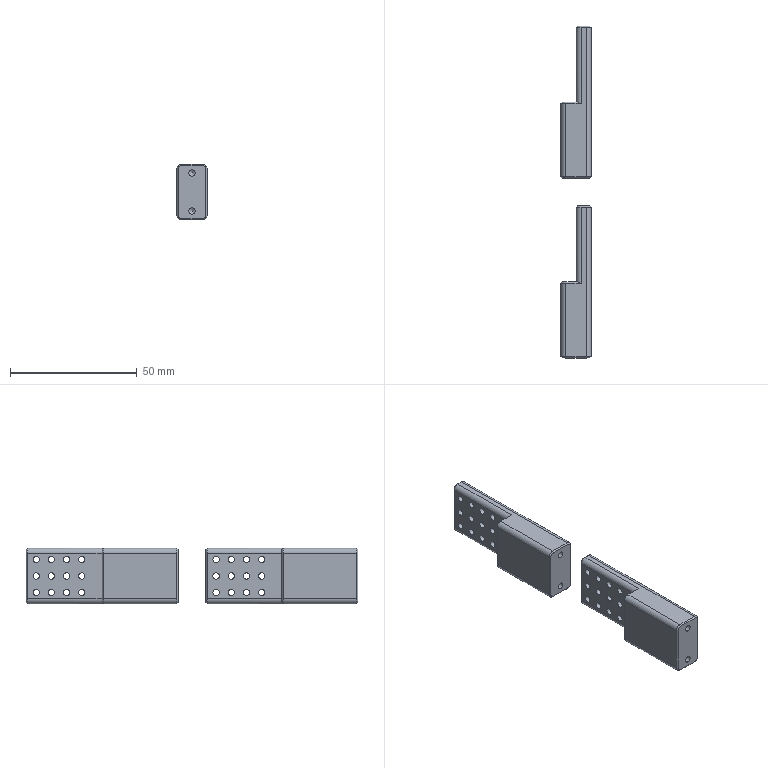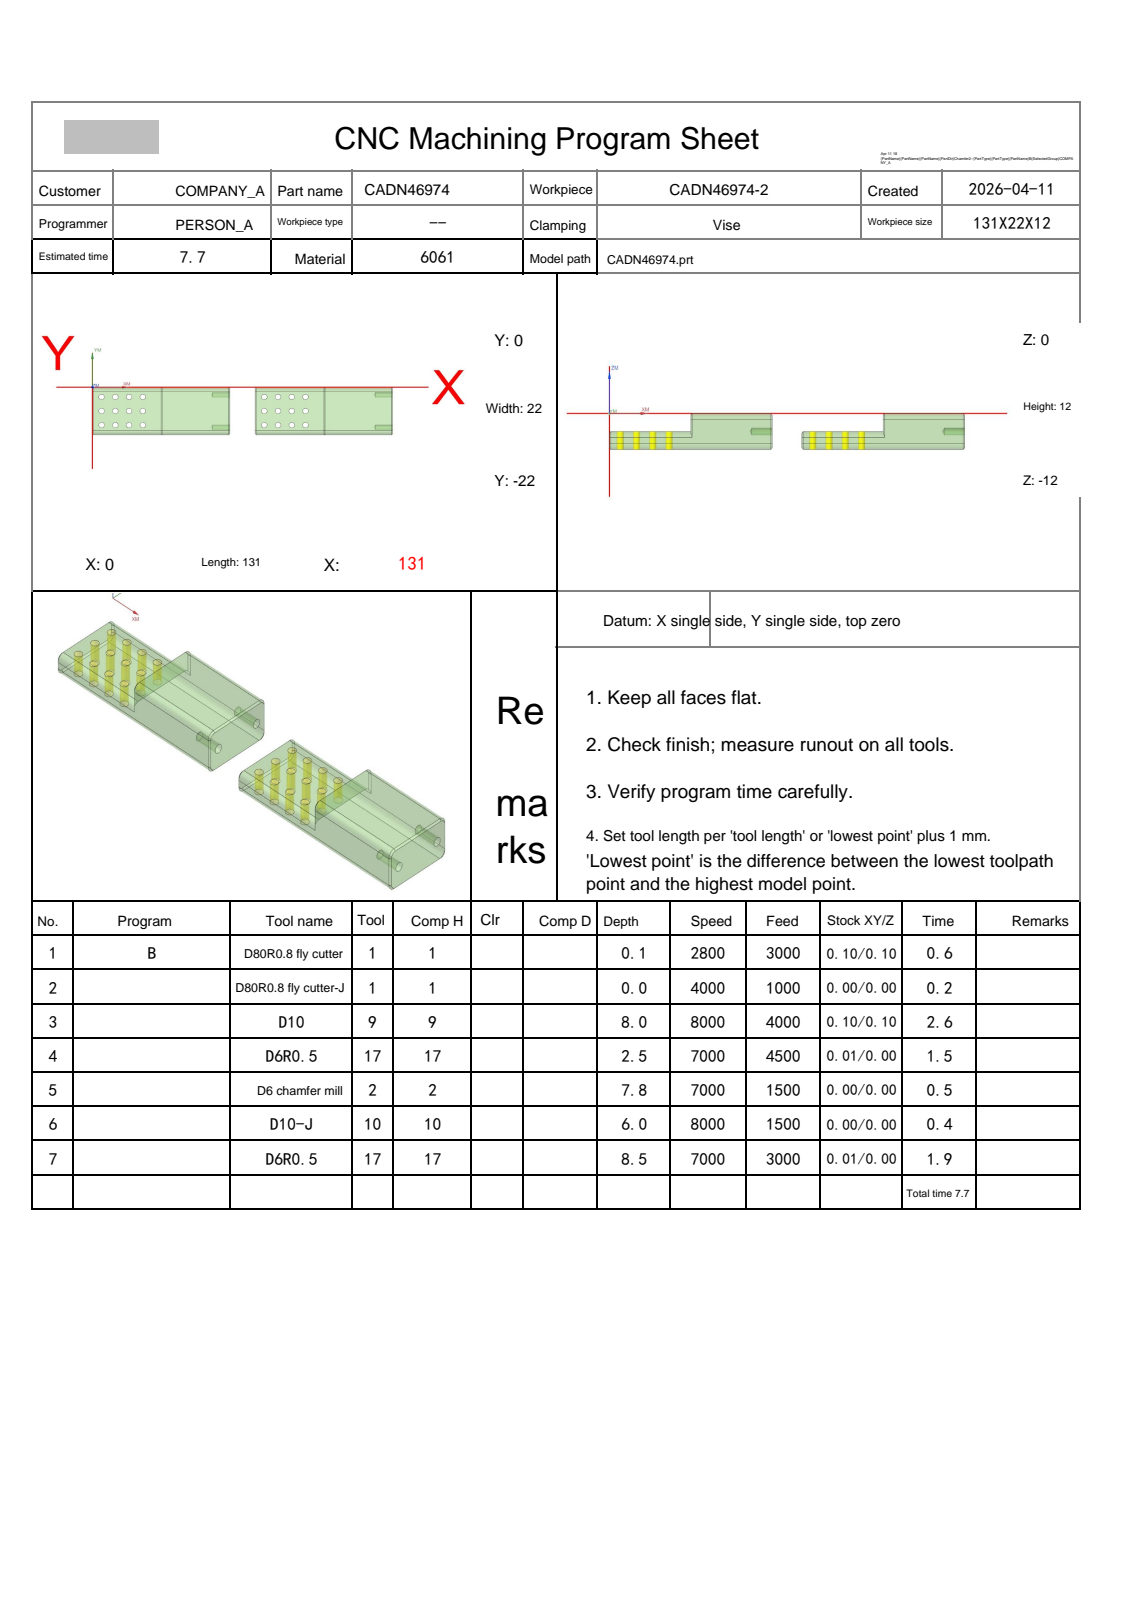NC program | NX | posted by the shop | part box 12 x 131 x 22 mm
Lines 2208 to 4050 of 5054, first 1531 of 1843 lines:
N4 T17 M06
(D6R0.5  D=6. R=0.5 H=17 ce=0.01 di=0.00)
G00 G90 G54 X134.304 Y-17.731 M03 S7000
G43 H17 Z12.8
M08
Z.491
G01 Z-.009 F4500.
X134.298
G03 X133.098 Y-18.901 I0.0 J-1.2
G01 X133.062 Y-20.314
X133.057 Y-20.363
G02 X130.5 Y-22.721 I-2.634 J.291
G01 X101.5
G02 X98.936 Y-20.411 I.115 J2.706
G01 X98.922 Y-20.314
X98.9 Y-18.897
X98.868 Y-18.899 Z-.015
X98.852 Y-18.9 Z-.021
X98.866 Y-20.229
G03 X101.5 Y-22.836 I2.634 J.027
G01 X130.5
G03 X133.136 Y-20.123 I-.105 J2.739
G01 X133.148 Y-18.824
X133.2 Y-18.862 Z-.038
G02 X133.221 Y-19.445 I-7.917 J-.583
X133.119 Y-20.718 I-7.939 J0.0
X130.503 Y-22.943 I-2.616 J.425
G01 X101.5
G02 X98.835 Y-20.462 I.099 J2.778
G01 X98.815 Y-20.314
X98.802 Y-18.898
X98.776 Y-18.9 Z-.048
X98.761 Y-18.901 Z-.058
X98.774 Y-20.314
X98.806 Y-20.574
G03 X101.5 Y-23.046 I2.795 J.343
G01 X130.5
G03 X133.183 Y-20.659 I-.1 J2.813
G01 X133.227 Y-20.314
X133.239 Y-18.893
X133.284 Y-18.849 Z-.082
G02 X133.307 Y-19.453 I-7.772 J-.604
X133.185 Y-20.829 I-7.795 J0.0
X130.5 Y-23.147 I-2.772 J.497
G01 X101.5
G02 X98.773 Y-20.659 I.093 J2.84
G01 X98.729 Y-20.314
X98.717 Y-18.898
X98.695 Y-18.899 Z-.096
X98.682 Z-.111
X98.691 Y-20.217
G03 X98.884 Y-21.265 I3.067 J.022
G01 X98.979 Y-21.52
G03 X101.5 Y-23.245 I2.589 J1.078
G01 X130.5
X131.427 Y-23.074
G03 X133.307 Y-20.314 I-1.159 J2.809
G01 X133.321 Y-18.887
X133.358 Y-18.914 Z-.143
X133.341 Y-20.314
X133.309 Y-20.659
G02 X131.734 Y-23.033 I-3.07 J.327
X130.5 Y-23.342 I-1.431 J3.097
G01 X101.499
G02 X99.343 Y-22.252 I0.0 J2.678
X98.654 Y-20.314 I2.867 J2.111
G01 X98.642 Y-18.9
X98.605 Y-18.892 Z-.178
X98.614 Y-20.143
G03 X98.98 Y-21.785 I4.005 J.03
X101.5 Y-23.437 I2.578 J1.184
G01 X130.542
G03 X132.379 Y-22.673 I0.0 J2.591
X133.379 Y-20.314 I-2.438 J2.424
G01 X133.395 Y-18.879
X133.435 Y-18.87 Z-.218
X133.42 Y-20.314
X133.385 Y-20.659
G02 X132.434 Y-22.729 I-3.452 J.333
X130.5 Y-23.53 I-1.994 J2.08
G01 X101.5
G02 X99.052 Y-22.039 I.043 J2.826
X98.575 Y-20.171 I3.544 J1.899
G01 X98.565 Y-18.893
X98.522 Y-18.895 Z-.261
Y-19.969
Y-19.986
G03 X98.983 Y-22.039 I4.81 J0.0
X101.5 Y-23.622 I2.57 J1.295
G01 X130.5
G03 X133.008 Y-22.039 I-.042 J2.846
X133.466 Y-20.314 I-3.959 J1.972
G01 X133.478 Y-18.895
X133.524 Y-18.896 Z-.307
X133.512 Y-20.314
X133.476 Y-20.659
G02 X132.873 Y-22.384 I-4.307 J.538
X130.5 Y-23.711 I-2.397 J1.502
G01 X101.5
G02 X98.979 Y-22.133 I.036 J2.86
X98.476 Y-19.978 I4.359 J2.154
G01 Y-19.969
Y-18.896
X98.425 Y-18.897 Z-.357
Y-19.969
G03 X99.063 Y-22.384 I4.888 J0.0
X101.5 Y-23.798 I2.461 J1.435
G01 X130.5
G03 X132.945 Y-22.384 I-.043 J2.894
X133.575 Y-19.969 I-4.383 J2.433
G01 Y-18.897
X133.628 Y-18.899 Z-.411
G02 X133.636 Y-19.434 I-17.574 J-.535
X133.623 Y-20.105 I-17.582 J0.0
X132.993 Y-22.39 I-5.175 J.198
X130.5 Y-23.883 I-2.517 J1.375
G01 X101.5
G02 X98.995 Y-22.379 I.033 J2.893
X98.382 Y-20.029 I4.383 J2.398
G01 X98.372 Y-18.934
Y-18.899
X98.315 Y-18.901 Z-.468
G03 X98.307 Y-19.433 I17.643 J-.533
X98.321 Y-20.132 I17.651 J0.0
X99.153 Y-22.729 I5.098 J.202
X101.5 Y-23.966 I2.378 J1.667
G01 X130.5
G03 X132.939 Y-22.592 I-.037 J2.917
G01 X133.052 Y-22.384
G03 X133.665 Y-20.325 I-4.423 J2.438
X133.698 Y-19.448 I-11.669 J.877
X133.685 Y-18.901 I-11.702 J0.0
G01 X133.745 Y-18.902 Z-.528
G02 X133.758 Y-19.447 I-11.605 J-.544
X133.729 Y-20.266 I-11.618 J0.0
X132.912 Y-22.719 I-5.196 J.367
X130.5 Y-24.047 I-2.435 J1.568
G01 X101.5
G02 X99.097 Y-22.729 I.02 J2.886
X98.305 Y-20.659 I4.593 J2.943
X98.242 Y-19.439 I11.682 J1.22
X98.255 Y-18.888 I11.745 J0.0
G01 X98.192 Y-18.895 Z-.591
G03 X98.184 Y-19.367 I13.801 J-.472
X98.244 Y-20.659 I13.809 J0.0
X99.134 Y-22.873 I5.506 J.927
X101.498 Y-24.125 I2.365 J1.609
G01 X130.502
G03 X132.851 Y-22.893 I0.0 J2.856
X133.757 Y-20.659 I-4.549 J3.146
X133.821 Y-19.437 I-11.656 J1.222
X133.808 Y-18.895 I-11.72 J0.0
G01 X133.874 Y-18.857 Z-.658
G02 X133.882 Y-19.35 I-14.17 J-.493
X133.822 Y-20.659 I-14.179 J0.0
X133.016 Y-22.729 I-5.538 J.965
G01 X132.783 Y-23.074
G02 X130.5 Y-24.2 I-2.308 J1.802
G01 X101.5
G02 X99.221 Y-23.074 I.016 J2.902
X98.18 Y-20.659 I4.483 J3.364
X98.118 Y-19.371 I13.177 J1.288
X98.126 Y-18.893 I13.24 J0.0
G01 X98.06 Y-18.873 Z-.727
G03 X98.049 Y-19.388 I12.491 J-.515
X98.114 Y-20.659 I12.502 J0.0
X98.979 Y-22.807 I5.655 J1.029
G01 X99.153 Y-23.074
G03 X101.5 Y-24.272 I2.375 J1.755
G01 X130.503
G03 X132.896 Y-22.989 I0.0 J2.874
G01 X133.069 Y-22.729
G03 X133.888 Y-20.659 I-4.561 J3.001
X133.95 Y-19.394 I-12.75 J1.266
X133.937 Y-18.818 I-12.813 J0.0
G01 X134.01 Y-18.851 Z-.798
G02 X134.021 Y-19.375 I-12.518 J-.524
X133.955 Y-20.659 I-12.529 J0.0
X133.114 Y-22.744 I-5.292 J.923
X131.746 Y-24.054 I-2.75 J1.503
X130.513 Y-24.341 I-1.233 J2.508
G01 X101.5
G02 X99.101 Y-23.074 I.02 J2.943
G01 X98.979 Y-22.886
X98.872 Y-22.729
G02 X98.046 Y-20.659 I4.544 J3.013
X97.979 Y-19.392 I11.911 J1.267
X97.993 Y-18.807 I11.978 J0.0
G01 X97.916 Y-18.922 Z-.868
G03 X97.908 Y-19.353 I12.331 J-.432
X97.978 Y-20.659 I12.339 J0.0
X98.979 Y-22.965 I5.452 J.997
X101.5 Y-24.404 I2.547 J1.533
G01 X130.512
G03 X132.403 Y-23.687 I0.0 J2.85
X133.177 Y-22.729 I-2.47 J2.787
X134.022 Y-20.659 I-4.327 J2.975
X134.091 Y-19.376 I-11.896 J1.283
X134.075 Y-18.762 I-11.965 J0.0
G01 X134.119 Y-18.843 Z-.904
X134.155 Y-18.924 Z-.939
X134.148 Y-19.969
G02 X133.631 Y-22.039 I-4.64 J.061
X132.773 Y-23.373 I-6.825 J3.448
X130.503 Y-24.463 I-2.27 J1.819
G01 X101.5
G02 X98.979 Y-23.044 I.038 J3.016
X97.91 Y-20.659 I4.625 J3.506
X97.838 Y-19.335 I12.252 J1.324
X97.845 Y-18.924 I12.324 J0.0
G01 X97.809 Y-18.925 Z-.974
X97.775 Y-18.926 Z-1.01
X97.781 Y-19.969
G03 X98.289 Y-22.007 I4.711 J.094
X99.212 Y-23.419 I7.675 J4.006
X101.5 Y-24.517 I2.303 J1.865
G01 X130.5
G03 X132.769 Y-23.442 I-.024 J2.981
X133.691 Y-22.039 I-6.854 J5.512
X134.219 Y-19.969 I-4.136 J2.156
G01 X134.226 Y-18.926
X134.261 Y-18.927 Z-1.045
X134.296 Y-18.928 Z-1.08
X134.289 Y-19.969
G02 X133.752 Y-22.039 I-4.66 J.105
X132.769 Y-23.495 I-8.012 J4.352
X130.5 Y-24.568 I-2.285 J1.895
G01 X101.495
G02 X99.253 Y-23.52 I0.0 J2.924
X98.289 Y-22.119 I6.943 J5.805
X97.712 Y-19.969 I4.069 J2.246
G01 X97.704 Y-18.928
X97.668 Y-18.929 Z-1.116
X97.633 Y-18.93 Z-1.151
X97.642 Y-19.969
G03 X98.19 Y-22.039 I4.546 J.095
X99.302 Y-23.621 I7.794 J4.297
X101.499 Y-24.615 I2.198 J1.934
G01 X130.5
G03 X132.769 Y-23.547 I-.023 J2.994
G01 X132.873 Y-23.419
G03 X133.803 Y-22.053 I-7.135 J5.857
X134.359 Y-19.969 I-4.069 J2.202
G01 X134.367 Y-18.93
X134.403 Y-18.931 Z-1.186
X134.438 Y-18.932 Z-1.222
X134.43 Y-19.969
G02 X133.868 Y-22.039 I-4.516 J.115
X132.616 Y-23.764 I-8.164 J4.607
X130.5 Y-24.659 I-2.143 J2.12
G01 X101.5
G02 X99.384 Y-23.764 I.021 J3.
X98.133 Y-22.039 I7.133 J6.49
X97.573 Y-19.969 I3.897 J2.165
G01 X97.562 Y-18.932
X97.527 Y-18.933 Z-1.257
X97.492 Y-18.934 Z-1.293
X97.503 Y-19.969
G03 X98.076 Y-22.039 I4.373 J.097
X99.408 Y-23.833 I8.913 J5.226
X101.048 Y-24.662 I2.114 J2.144
G01 X101.5 Y-24.699
X130.5
G03 X132.658 Y-23.764 I-.031 J3.03
X133.924 Y-22.039 I-7.483 J6.819
X134.5 Y-19.969 I-3.83 J2.181
G01 X134.509 Y-18.934
X134.543 Y-19.083 Z-1.328
X134.576 Y-19.231 Z-1.363
X134.571 Y-19.969
G02 X133.98 Y-22.039 I-4.306 J.11
X132.769 Y-23.676 I-8.71 J5.18
G01 X132.696 Y-23.764
G02 X131.045 Y-24.684 I-2.21 J2.023
G01 X130.5 Y-24.737
X101.5
X101.048 Y-24.701
G02 X99.306 Y-23.764 I.46 J2.943
X98.125 Y-22.219 I9.01 J8.108
X97.455 Y-20.277 I3.641 J2.344
X97.42 Y-19.527 I8.026 J.75
X97.425 Y-19.228 I8.061 J0.0
G01 X97.409 Y-19.397 Z-1.381
X97.393 Y-19.566 Z-1.399
X97.377 Y-19.734 Z-1.416
X97.363 Y-19.903 Z-1.434
G03 X97.945 Y-22.006 I4.116 J.007
X99.275 Y-23.764 I9.42 J5.749
G01 X99.324 Y-23.824
G03 X101.5 Y-24.771 I2.188 J2.052
G01 X130.5
G03 X132.728 Y-23.764 I-.014 J2.998
G01 X132.769 Y-23.715
G03 X134.036 Y-22.039 I-7.98 J7.352
X134.641 Y-19.922 I-3.575 J2.168
G01 X134.649 Y-20.076 Z-1.444
X134.646 Y-20.229 Z-1.455
X134.639 Y-20.383 Z-1.465
X134.63 Y-20.537 Z-1.476
X134.614 Y-20.69 Z-1.486
X134.59 Y-20.84 Z-1.496
X134.559 Y-20.988 Z-1.507
G02 X134.094 Y-22.039 I-4.048 J1.163
X132.595 Y-23.936 I-10.144 J6.475
X130.5 Y-24.804 I-2.104 J2.115
G01 X101.5
G02 X99.301 Y-23.833 I.013 J3.004
G01 X99.244 Y-23.764
G02 X97.945 Y-22.101 I8.56 J8.028
X97.441 Y-20.991 I3.59 J2.297
G01 X97.462 Y-21.129 Z-1.526
X97.49 Y-21.264 Z-1.545
X97.527 Y-21.397 Z-1.565
X97.571 Y-21.525 Z-1.584
G03 X97.945 Y-22.196 I3.829 J1.693
X98.902 Y-23.419 I10.343 J7.104
G01 X99.211 Y-23.764
X99.268 Y-23.833
G03 X101.5 Y-24.836 I2.243 J2.008
G01 X130.5
G03 X132.612 Y-23.954 I-.008 J2.986
X134.148 Y-22.049 I-9.472 J9.214
X134.43 Y-21.521 I-2.751 J1.811
G01 X134.402 Y-21.64 Z-1.611
X134.366 Y-21.757 Z-1.639
X134.316 Y-21.865 Z-1.666
X134.148 Y-22.148
G02 X132.63 Y-23.973 I-13.4 J9.608
X130.5 Y-24.867 I-2.14 J2.115
G01 X101.495
G02 X99.378 Y-23.976 I0.0 J2.959
X97.945 Y-22.278 I11.005 J10.749
X97.68 Y-21.866 I2.727 J2.042
G01 X97.719 Y-21.994 Z-1.709
X97.771 Y-22.114 Z-1.751
G03 X99.04 Y-23.651 I11.128 J7.893
G01 X99.28 Y-23.902
X99.324 Y-23.957
G03 X101.5 Y-24.895 I2.194 J2.095
G01 X130.501
G03 X132.7 Y-23.926 I0.0 J2.981
G01 X132.769 Y-23.852
G03 X134.226 Y-22.12 I-11.388 J11.064
G01 X134.19 Y-22.222 Z-1.796
X134.146 Y-22.317 Z-1.84
G02 X132.769 Y-23.879 I-16.258 J12.952
G01 X132.658 Y-24.001
G02 X130.5 Y-24.921 I-2.167 J2.092
G01 X101.5
G02 X99.311 Y-23.971 I.008 J3.014
G01 X99.254 Y-23.902
G02 X97.849 Y-22.304 I11.657 J11.671
G01 X97.914 Y-22.46 Z-1.931
G03 X99.227 Y-23.902 I22.34 J19.019
G01 X99.288 Y-23.971
G03 X101.5 Y-24.944 I2.221 J2.048
G01 X130.5
G03 X132.671 Y-24.015 I-.016 J3.036
G01 X132.769 Y-23.906
G03 X134.099 Y-22.444 I-20.932 J20.375
G01 X134.058 Y-22.542 Z-2.025
G02 X132.68 Y-24.025 I-27.765 J24.408
X130.5 Y-24.964 I-2.186 J2.072
G01 X101.5
G02 X99.334 Y-24.04 I.004 J3.008
X97.96 Y-22.569 I34.655 J33.753
G01 X97.997 Y-22.654 Z-2.121
G03 X99.384 Y-24.109 I47.473 J43.852
X101.5 Y-24.981 I2.122 J2.145
G01 X130.503
G03 X132.631 Y-24.093 I0.0 J2.994
X134.011 Y-22.638 I-34.23 J33.868
G01 X133.963 Y-22.729 Z-2.216
G02 X132.58 Y-24.158 I-81.21 J77.228
X130.5 Y-24.994 I-2.097 J2.213
G01 X101.5
G02 X99.303 Y-24.04 I.013 J3.036
G01 X98.036 Y-22.731
X98.044 Y-22.762 Z-2.311
X99.376 Y-24.122
G03 X99.925 Y-24.556 I1.98 J1.94
X101.5 Y-25.003 I1.607 J2.664
G01 X130.5
G03 X132.587 Y-24.158 I-.018 J3.045
G01 X132.769 Y-23.972
X133.949 Y-22.765
X133.933 Y-22.798 Z-2.405
X132.636 Y-24.116
G02 X130.506 Y-25.008 I-2.13 J2.097
G01 X101.499
G02 X99.362 Y-24.114 I0.0 J3.001
G01 X98.289 Y-23.027
X98.056 Y-22.789
X98.069 Y-22.815 Z-2.5
X98.289 Y-23.041
X99.352 Y-24.109
G03 X101.5 Y-25.01 I2.149 J2.112
G01 X130.5
G03 X132.598 Y-24.158 I0.0 J3.01
G01 X132.769 Y-23.988
X133.917 Y-22.831
G00 Z12.8
X97.696 Y-4.284
Z.491
G01 Z-.009
X97.7
G03 X98.9 Y-3.103 I0.0 J1.2
G01 X98.922 Y-1.686
X98.936 Y-1.589
G02 X101.5 Y.721 I2.679 J-.396
G01 X130.5
G02 X133.041 Y-1.768 I-.05 J-2.593
G01 X133.1 Y-3.238
X133.148 Y-3.1 Z-.021
X133.136 Y-1.877
G03 X130.5 Y.836 I-2.741 J-.027
G01 X101.5
G03 X98.881 Y-1.545 I.08 J-2.719
G01 X98.867 Y-1.686
X98.852 Y-3.099
X98.801 Y-3.1 Z-.038
X98.815 Y-1.686
X98.835 Y-1.538
G02 X101.5 Y.943 I2.764 J-.297
G01 X130.505
G02 X133.117 Y-1.274 I0.0 J-2.648
X133.221 Y-2.536 I-7.65 J-1.263
X133.2 Y-3.1 I-7.753 J0.0
G01 X133.223 Z-.048
X133.239 Z-.058
X133.227 Y-1.686
X133.183 Y-1.341
G03 X130.5 Y1.046 I-2.783 J-.427
G01 X101.5
G03 X98.804 Y-1.436 I.111 J-2.826
G01 X98.774 Y-1.686
X98.761 Y-3.099
X98.734 Y-3.1 Z-.07
X98.717 Y-3.102 Z-.082
X98.729 Y-1.686
X98.773 Y-1.341
G02 X101.5 Y1.147 I2.819 J-.352
G01 X130.5
G02 X133.184 Y-1.161 I-.087 J-2.816
X133.307 Y-2.516 I-7.385 J-1.356
X133.285 Y-3.1 I-7.508 J0.0
G01 X133.321 Z-.111
X133.307 Y-1.686
X133.271 Y-1.341
G03 X130.5 Y1.245 I-2.885 J-.314
G01 X101.5
G03 X100.013 Y.781 I.106 J-2.953
X98.719 Y-1.424 I1.776 J-2.524
G01 X98.692 Y-1.686
X98.682 Y-3.101
X98.658 Y-3.1 Z-.127
X98.642 Z-.143
X98.654 Y-1.686
X98.687 Y-1.341
G02 X100.358 Y1.084 I3.104 J-.351
X101.5 Y1.342 I1.417 J-3.623
G01 X130.5
G02 X132.813 Y.039 I-.062 J-2.815
G01 X132.938 Y-.191
G02 X133.341 Y-1.742 I-2.947 J-1.595
G01 X133.359 Y-3.1
X133.395 Y-3.121 Z-.178
X133.379 Y-1.686
G03 X132.883 Y.039 I-3.682 J-.123
X130.5 Y1.437 I-2.445 J-1.438
G01 X101.5
G03 X99.673 Y.729 I.087 J-2.938
X98.65 Y-1.341 I2.328 J-2.438
G01 X98.615 Y-1.686
X98.605 Y-3.108
X98.565 Y-3.107 Z-.218
X98.576 Y-1.686
X98.613 Y-1.341
G02 X99.221 Y.31 I3.757 J-.447
X101.5 Y1.53 I2.279 J-1.518
G01 X130.5
G02 X133.12 Y-.306 I-.063 J-2.878
X133.433 Y-1.992 I-4.391 J-1.686
G01 Y-2.031
X133.435 Y-3.13
X133.478 Y-3.106 Z-.261
X133.466 Y-1.686
G03 X133.008 Y.039 I-4.416 J-.247
X130.5 Y1.622 I-2.55 J-1.263
G01 X101.5
G03 X98.983 Y.039 I.052 J-2.877
X98.532 Y-1.904 I4.126 J-1.981
G01 X98.522 Y-3.105
X98.499 Z-.284
X98.476 Y-3.104 Z-.307
X98.486 Y-1.917
G02 X98.976 Y.127 I4.67 J-.04
X101.5 Y1.711 I2.56 J-1.276
G01 X130.5
G02 X133.067 Y.039 I-.037 J-2.865
X133.524 Y-2.027 I-4.442 J-2.066
G01 Y-2.031
Y-3.105
X133.575 Y-3.103 Z-.357
Y-2.031
G03 X132.945 Y.384 I-5.013 J-.018
X130.5 Y1.798 I-2.487 J-1.48
G01 X101.5
G03 X99.063 Y.384 I.024 J-2.849
X98.438 Y-1.686 I4.231 J-2.407
G01 X98.425 Y-3.103
X98.399 Y-3.102 Z-.384
X98.372 Y-3.101 Z-.411
G02 X98.364 Y-2.566 I18.376 J.535
X98.378 Y-1.861 I18.384 J0.0
X98.992 Y.374 I5.078 J-.195
X101.5 Y1.883 I2.541 J-1.383
G01 X130.5
G02 X132.993 Y.39 I-.024 J-2.868
X133.623 Y-1.897 I-4.546 J-2.483
X133.636 Y-2.568 I-17.763 J-.671
X133.628 Y-3.102 I-17.776 J0.0
G01 X133.685 Y-3.1 Z-.468
G03 X133.698 Y-2.55 I-11.598 J.55
X133.665 Y-1.67 I-11.611 J0.0
X133.069 Y.352 I-5.028 J-.382
G01 X132.939 Y.592
G03 X130.5 Y1.966 I-2.476 J-1.542
G01 X101.5
G03 X99.153 Y.729 I.031 J-2.904
X98.321 Y-1.866 I4.267 J-2.799
X98.307 Y-2.565 I17.476 J-.699
X98.315 Y-3.099 I17.49 J0.0
G01 X98.255 Y-3.112 Z-.528
G02 X98.242 Y-2.566 I11.922 J.545
X98.305 Y-1.341 I11.935 J0.0
X99.097 Y.729 I5.385 J-.873
X101.5 Y2.047 I2.423 J-1.569
G01 X130.5
G02 X132.912 Y.719 I-.022 J-2.896
X133.729 Y-1.732 I-4.382 J-2.822
X133.758 Y-2.55 I-11.474 J-.818
X133.745 Y-3.098 I-11.503 J0.0
G01 X133.808 Y-3.105 Z-.591
G03 X133.822 Y-2.557 I-11.482 J.549
X133.757 Y-1.341 I-11.495 J0.0
X132.851 Y.893 I-5.455 J-.913
X130.502 Y2.125 I-2.349 J-1.625
G01 X101.499
G03 X99.133 Y.873 I0.0 J-2.86
X98.244 Y-1.341 I4.618 J-3.141
X98.184 Y-2.636 I13.839 J-1.295
X98.192 Y-3.105 I13.899 J0.0
G01 X98.126 Y-3.085 Z-.658
G02 X98.118 Y-2.627 I13.249 J.458
X98.18 Y-1.341 I13.257 J0.0
X99.221 Y1.074 I5.526 J-.951
X101.5 Y2.2 I2.295 J-1.776
G01 X130.5
G02 X132.783 Y1.074 I-.025 J-2.928
G01 X132.948 Y.83
G02 X133.822 Y-1.341 I-4.634 J-3.127
X133.881 Y-2.632 I-13.939 J-1.291
X133.874 Y-3.086 I-13.999 J0.0
G01 X133.909 Y-3.085 Z-.692
X133.942 Y-3.084 Z-.727
G03 X133.95 Y-2.625 I-13.192 J.458
X133.888 Y-1.341 I-13.2 J0.0
X133.069 Y.729 I-5.378 J-.93
G01 X132.84 Y1.074
G03 X130.5 Y2.272 I-2.357 J-1.72
G01 X101.498
G03 X99.079 Y.961 I0.0 J-2.887
G01 X98.979 Y.807
G03 X98.114 Y-1.341 I4.793 J-3.179
X98.049 Y-2.627 I12.735 J-1.286
X98.057 Y-3.083 I12.799 J0.0
G01 X98.021 Y-3.082 Z-.762
X97.986 Y-3.081 Z-.798
G02 X97.978 Y-2.635 I12.478 J.446
X98.046 Y-1.341 I12.486 J0.0
X98.979 Y.886 I5.399 J-.954
X101.5 Y2.341 I2.545 J-1.498
G01 X130.5
G02 X132.898 Y1.074 I-.019 J-2.939
X133.666 Y-.306 I-5.847 J-4.159
X134.01 Y-2.031 I-4.323 J-1.76
G01 X134.013 Y-3.081
X134.049 Y-3.08 Z-.833
X134.084 Y-3.079 Z-.868
X134.079 Y-1.991
G03 X133.741 Y-.336 I-4.302 J-.017
X132.769 Y1.316 I-6.67 J-2.813
X130.5 Y2.404 I-2.287 J-1.861
G01 X101.5
G03 X98.979 Y.965 I.026 J-2.972
X97.977 Y-1.341 I4.456 J-3.306
X97.908 Y-2.645 I12.169 J-1.304
X97.915 Y-3.078 I12.238 J0.0
G01 X97.879 Y-3.077 Z-.904
X97.845 Y-3.076 Z-.939
G02 X97.838 Y-2.667 I12.329 J.409
X97.909 Y-1.341 I12.336 J0.0
X98.979 Y1.044 I5.699 J-1.125
X101.5 Y2.463 I2.559 J-1.597
G01 X130.503
G02 X132.773 Y1.373 I0.0 J-2.909
X133.631 Y.039 I-5.959 J-4.776
X134.149 Y-2.031 I-4.133 J-2.134
G01 X134.154 Y-3.077
X134.19 Y-3.076 Z-.974
X134.225 Y-3.074 Z-1.01
X134.218 Y-2.031
G03 X133.691 Y.039 I-4.666 J-.086
X132.769 Y1.442 I-7.764 J-4.1
X130.5 Y2.517 I-2.291 J-1.904
G01 X101.5
G03 X99.212 Y1.419 I.015 J-2.963
X98.289 Y.007 I6.754 J-5.42
X97.78 Y-2.031 I4.208 J-2.134
G01 X97.774 Y-3.074
X97.738 Y-3.073 Z-1.045
X97.703 Y-3.072 Z-1.08
X97.71 Y-2.031
G02 X98.289 Y.119 I4.658 J-.103
X99.25 Y1.516 I7.908 J-4.405
X101.498 Y2.568 I2.249 J-1.878
G01 X130.5
G02 X132.83 Y1.419 I-.014 J-2.967
X133.752 Y.039 I-7.044 J-5.701
X134.288 Y-2.031 I-4.117 J-2.171
G01 X134.296 Y-3.072
X134.331 Y-3.071 Z-1.116
X134.366 Y-3.07 Z-1.151
X134.358 Y-2.031
G03 X133.803 Y.053 I-4.611 J-.112
X132.721 Y1.6 I-8.049 J-4.479
X130.501 Y2.615 I-2.22 J-1.92
G01 X101.499
G03 X99.302 Y1.622 I0.0 J-2.926
X98.19 Y.039 I6.683 J-5.881
X97.641 Y-2.031 I4.012 J-2.172
G01 X97.632 Y-3.07
X97.597 Y-3.069 Z-1.186
X97.561 Y-3.068 Z-1.222
X97.57 Y-2.031
G02 X98.133 Y.039 I4.482 J-.107
X99.384 Y1.764 I8.387 J-4.767
X101.5 Y2.659 I2.133 J-2.095
G01 X130.5
G02 X132.616 Y1.764 I-.022 J-3.004
X133.867 Y.039 I-6.898 J-6.32
X134.427 Y-2.031 I-3.932 J-2.174
G01 X134.437 Y-3.067
X134.507 Y-3.032 Z-1.293
X134.497 Y-2.031
G03 X133.923 Y.039 I-4.372 J-.097
X132.602 Y1.823 I-8.638 J-5.018
X130.5 Y2.699 I-2.134 J-2.16
G01 X101.5
X101.048 Y2.662
G03 X99.408 Y1.833 I.465 J-2.957
X98.076 Y.039 I7.585 J-7.023
X97.499 Y-2.031 I3.838 J-2.185
G01 X97.491 Y-3.066
X97.456 Y-2.916 Z-1.328
X97.423 Y-2.767 Z-1.363
X97.428 Y-2.031
G02 X98.019 Y.039 I4.318 J-.114
X99.306 Y1.764 I9.597 J-5.818
X101.048 Y2.701 I2.203 J-2.008
G01 X101.5 Y2.737
X130.5
G02 X132.114 Y2.257 I-.043 J-3.101
X132.769 Y1.676 I-1.539 J-2.394
X133.973 Y.051 I-7.469 J-6.792
X134.539 Y-1.666 I-3.582 J-2.134
X134.58 Y-2.47 I-7.991 J-.803
X134.574 Y-2.762 I-8.032 J0.0
G01 X134.591 Y-2.598 Z-1.381
X134.606 Y-2.433 Z-1.399
X134.622 Y-2.268 Z-1.416
X134.637 Y-2.103 Z-1.434
G03 X134.035 Y.039 I-4.122 J-.001
X133.025 Y1.419 I-8.194 J-4.942
G01 X132.769 Y1.715
X132.728 Y1.764
G03 X130.5 Y2.771 I-2.24 J-1.988
G01 X101.5
G03 X99.401 Y1.902 I.018 J-3.013
X97.962 Y.039 I8.417 J-7.986
X97.357 Y-2.07 I3.611 J-2.177
G01 X97.351 Y-1.918 Z-1.444
X97.354 Y-1.764 Z-1.455
X97.361 Y-1.611 Z-1.465
X97.37 Y-1.458 Z-1.476
X97.386 Y-1.306 Z-1.486
X97.41 Y-1.156 Z-1.496
X97.441 Y-1.009 Z-1.507
G02 X97.945 Y.101 I4.098 J-1.19
X99.244 Y1.764 I9.862 J-6.367
G01 X99.301 Y1.833
G02 X101.5 Y2.804 I2.216 J-2.043
G01 X130.5
G02 X132.769 Y1.755 I-.017 J-3.013
G01 X133.06 Y1.419
G02 X134.008 Y.174 I-7.676 J-6.828
X134.558 Y-1.013 I-3.921 J-2.538
G01 X134.538 Y-.876 Z-1.526
X134.51 Y-.741 Z-1.545
X134.474 Y-.608 Z-1.565
X134.431 Y-.48 Z-1.584
G03 X133.972 Y.313 I-4.567 J-2.114
X132.671 Y1.894 I-11.564 J-8.184
X130.5 Y2.836 I-2.18 J-2.052
G01 X101.497
G03 X99.346 Y1.913 I0.0 J-2.968
X97.945 Y.196 I10.61 J-10.089
X97.571 Y-.475 I3.454 J-2.362
G01 X97.599 Y-.357 Z-1.611
X97.634 Y-.242 Z-1.639
X97.68 Y-.134 Z-1.666
G02 X98.018 Y.379 I4.893 J-2.858
X99.384 Y1.98 I12.24 J-9.059
X101.496 Y2.867 I2.112 J-2.07
G01 X130.5
G02 X132.631 Y1.971 I-.009 J-3.003
X134.034 Y.306 I-11.89 J-11.442
X134.318 Y-.139 I-3.227 J-2.374
G01 X134.28 Y-.008 Z-1.709
X134.229 Y.115 Z-1.751
G03 X132.852 Y1.764 I-12.609 J-9.131
G01 X132.769 Y1.852
X132.702 Y1.927
G03 X130.5 Y2.895 I-2.214 J-2.046
G01 X101.497
G03 X99.406 Y2.034 I0.0 J-2.968
X97.771 Y.114 I10.573 J-10.658
G01 X97.803 Y.214 Z-1.796
X97.849 Y.305 Z-1.84
G02 X99.254 Y1.902 I13.098 J-10.104
G01 X99.311 Y1.971
G02 X101.5 Y2.921 I2.196 J-2.062
G01 X130.504
G02 X132.769 Y1.879 I0.0 J-2.982
X134.148 Y.315 I-14.938 J-14.57
G01 X134.099 Y.444 Z-1.931
G03 X132.769 Y1.906 I-22.324 J-18.976
G01 X132.673 Y2.013
G03 X130.5 Y2.944 I-2.181 J-2.09
G01 X101.497
G03 X99.357 Y2.041 I0.0 J-2.986
X97.914 Y.46 I24.146 J-23.491
G01 X97.96 Y.569 Z-2.025
G02 X99.334 Y2.04 I36.234 J-32.47
X101.5 Y2.964 I2.17 J-2.085
G01 X130.5
G02 X132.598 Y2.109 I-.006 J-3.016
X134.058 Y.542 I-27.182 J-26.788
G01 X134.011 Y.64 Z-2.121
G03 X132.616 Y2.109 I-39.614 J-36.19
X130.5 Y2.981 I-2.124 J-2.15
G01 X101.5
G03 X99.384 Y2.109 I.007 J-3.02
X97.997 Y.654 I45.873 J-45.092
G01 X98.037 Y.73 Z-2.216
X99.167 Y1.902
X99.303 Y2.04
G02 X101.5 Y2.994 I2.208 J-2.08
G01 X130.5
G02 X132.63 Y2.109 I-.015 J-3.042
X133.963 Y.73 I-163.246 J-159.157
G01 X133.949 Y.765 Z-2.311
X132.64 Y2.109
G03 X130.5 Y3.003 I-2.161 J-2.167
G01 X101.5
X101.446 Y2.997
X101.435 Y2.998
G03 X99.365 Y2.109 I.054 J-2.982
G01 X99.296 Y2.04
X99.159 Y1.902
X98.045 Y.761
X98.056 Y.788 Z-2.405
X99.152 Y1.902
X99.377 Y2.129
G02 X101.496 Y3.008 I2.118 J-2.111
G01 X130.5
G02 X132.644 Y2.109 I-.009 J-3.028
G01 X133.933 Y.798
X133.917 Y.83 Z-2.5
X132.652 Y2.104
G03 X130.5 Y3.01 I-2.152 J-2.102
G01 X101.496
G03 X99.373 Y2.128 I0.0 J-2.996
G01 X98.289 Y1.04
X98.069 Y.814
G00 Z12.8
X63.304 Y-17.565
Z.491
G01 Z-.009
X63.303
X63.3
G03 X62.1 Y-18.762 I0.0 J-1.2
G01 X62.097 Y-19.969
Y-19.977
G02 X59.5 Y-22.721 I-2.748 J0.0
G01 X30.636
G02 X27.903 Y-19.989 I0.0 J2.733
G01 X27.902 Y-18.899
X27.868 Z-.015
X27.85 Z-.021
G03 X27.826 Y-19.46 I6.615 J-.561
X27.95 Y-20.74 I6.638 J0.0
X30.499 Y-22.836 I2.548 J.501
G01 X59.5
G03 X62.051 Y-20.721 I0.0 J2.596
X62.177 Y-19.369 I-7.176 J1.352
X62.152 Y-18.762 I-7.302 J0.0
G01 X62.179 Z-.03
X62.196 Z-.038
X62.183 Y-20.314
X62.122 Y-20.659
G02 X59.5 Y-22.943 I-2.706 J.459
G01 X30.5
G02 X27.878 Y-20.659 I.084 J2.743
G01 X27.817 Y-20.314
X27.804 Y-18.898
X27.776 Y-18.899 Z-.048
X27.758 Z-.058
X27.773 Y-20.314
X27.817 Y-20.659
G03 X30.5 Y-23.046 I2.785 J.429
G01 X59.5
G03 X62.183 Y-20.659 I-.102 J2.816
G01 X62.227 Y-20.314
X62.243 Y-18.762
X62.28 Y-18.773 Z-.082
X62.27 Y-20.314
X62.227 Y-20.659
G02 X59.5 Y-23.147 I-2.822 J.356
G01 X30.5
G02 X27.85 Y-21.004 I.074 J2.802
X27.696 Y-19.494 I7.332 J1.51
X27.719 Y-18.899 I7.486 J0.0
G01 X27.695 Z-.096
X27.68 Y-18.9 Z-.111
G03 X27.657 Y-19.503 I7.894 J-.604
X27.78 Y-20.894 I7.917 J0.0
X30.5 Y-23.245 I2.809 J.501
G01 X59.5
G03 X62.27 Y-20.659 I-.14 J2.927
G01 X62.308 Y-20.314
X62.32 Y-18.786
X62.359 Y-18.897 Z-.143
X62.349 Y-20.314
X62.309 Y-20.659
G02 X59.5 Y-23.342 I-2.936 J.263
G01 X30.5
G02 X27.913 Y-21.508 I.082 J2.857
X27.641 Y-20.037 I3.839 J1.47
G01 X27.642 Y-19.969
X27.641 Y-18.906
X27.605 Y-18.887 Z-.178
X27.615 Y-20.153
G03 X28.012 Y-21.847 I3.947 J.031
X30.5 Y-23.437 I2.541 J1.235
G01 X59.5
G03 X61.325 Y-22.729 I-.08 J2.914
X62.341 Y-20.71 I-2.308 J2.427
X62.408 Y-19.447 I-11.925 J1.263
X62.395 Y-18.891 I-11.992 J0.0
G01 X62.435 Z-.218
G02 X62.452 Y-19.473 I-9.651 J-.582
X62.341 Y-20.933 I-9.669 J0.0
X60.979 Y-23.09 I-3.187 J.503
X59.56 Y-23.53 I-1.42 J2.07
G01 X30.5
G02 X28.049 Y-22.038 I.047 J2.836
X27.576 Y-20.193 I3.489 J1.878
G01 X27.565 Y-18.898
X27.522 Y-18.895 Z-.261
X27.523 Y-19.969
Y-20.022
G03 X28.005 Y-22.077 I4.619 J0.0
X30.5 Y-23.622 I2.54 J1.315
G01 X59.5
G03 X61.995 Y-22.077 I-.045 J2.86
X62.466 Y-20.314 I-4.033 J2.022
G01 X62.478 Y-18.902
X62.524 Z-.307
X62.512 Y-20.314
G02 X61.995 Y-22.179 I-4.732 J.309
X59.5 Y-23.711 I-2.528 J1.32
G01 X30.5
G02 X28.005 Y-22.179 I.033 J2.851
X27.476 Y-19.993 I4.249 J2.186
G01 Y-19.969
Y-18.895
X27.425 Y-18.897 Z-.357
X27.426 Y-19.969
G03 X28.005 Y-22.289 I4.957 J.006
X30.5 Y-23.798 I2.525 J1.358
G01 X59.5
G03 X61.995 Y-22.289 I-.031 J2.867
X62.574 Y-19.969 I-4.377 J2.326
G01 X62.575 Y-18.902
X62.628 Z-.411
X62.615 Y-20.314
G02 X61.995 Y-22.401 I-5.192 J.407
X59.5 Y-23.883 I-2.53 J1.418
G01 X30.5
G02 X28.005 Y-22.401 I.035 J2.9
X27.385 Y-20.314 I4.572 J2.494
G01 X27.372 Y-18.902
X27.315 Y-18.909 Z-.468
G03 X27.307 Y-19.438 I17.555 J-.529
X27.318 Y-20.068 I17.563 J0.0
X28.068 Y-22.592 I5.262 J.189
X30.497 Y-23.966 I2.429 J1.46
G01 X59.5
G03 X61.906 Y-22.634 I0.0 J2.838
X62.679 Y-20.127 I-4.326 J2.708
X62.693 Y-19.436 I-17.54 J.692
X62.685 Y-18.902 I-17.554 J0.0
G01 X62.745 Y-18.891 Z-.528
Y-19.624
X62.744 Y-19.969
G02 X62.105 Y-22.384 I-5.221 J.091
G01 X62.036 Y-22.515
G02 X59.501 Y-24.047 I-2.535 J1.332
G01 X30.5
G02 X28.005 Y-22.593 I.03 J2.919
G01 X27.895 Y-22.384
G02 X27.256 Y-19.969 I4.582 J2.506
G01 X27.255 Y-19.624
Y-18.891
X27.192 Y-18.898 Z-.591
G03 X27.184 Y-19.368 I13.678 J-.47
X27.245 Y-20.659 I13.686 J0.0
X28.036 Y-22.729 I5.575 J.945
X30.5 Y-24.125 I2.493 J1.529
G01 X59.5
G03 X61.964 Y-22.729 I-.029 J2.924
X62.755 Y-20.659 I-4.784 J3.015
X62.816 Y-19.364 I-13.777 J1.296
X62.808 Y-18.898 I-13.838 J0.0
G01 X62.874 Y-18.918 Z-.658
G02 X62.882 Y-19.372 I-13.226 J-.455
X62.819 Y-20.659 I-13.234 J0.0
X61.829 Y-23.009 I-5.61 J.982
X59.501 Y-24.2 I-2.328 J1.679
G01 X30.499
G02 X28.171 Y-23.009 I0.0 J2.87
X27.181 Y-20.659 I4.619 J3.331
X27.118 Y-19.365 I13.405 J1.295
X27.126 Y-18.915 I13.467 J0.0
G01 X27.091 Y-18.916 Z-.692
X27.057 Y-18.917 Z-.727
X27.059 Y-19.95
G03 X27.475 Y-21.881 I4.72 J.008
X28.124 Y-23.029 I6.599 J2.973
X30.498 Y-24.272 I2.374 J1.644
G01 X59.5
G03 X61.844 Y-23.074 I-.024 J2.938
X62.448 Y-22.039 I-5.241 J3.751
G01 X62.52 Y-21.882
G03 X62.941 Y-19.961 I-4.231 J1.934
G01 X62.944 Y-18.934
X62.94 Y-18.861
X63.007 Y-18.802 Z-.798
G02 X63.021 Y-19.38 I-12.29 J-.578
X62.954 Y-20.659 I-12.304 J0.0
X61.995 Y-22.936 I-5.555 J1.001
G01 X61.897 Y-23.074
G02 X59.5 Y-24.341 I-2.415 J1.668
G01 X30.5
G02 X28.103 Y-23.074 I.017 J2.935
G01 X28.005 Y-22.936
G02 X27.046 Y-20.659 I4.593 J3.277
X26.978 Y-19.377 I12.144 J1.283
X26.987 Y-18.919 I12.211 J0.0
G01 X26.951 Y-18.92 Z-.833
X26.916 Y-18.922 Z-.868
X26.919 Y-19.893
G03 X27.378 Y-21.935 I4.846 J.016
X28.242 Y-23.322 I6.247 J2.93
X30.497 Y-24.404 I2.255 J1.809
G01 X59.502
G03 X61.757 Y-23.323 I0.0 J2.893
X62.62 Y-21.938 I-5.336 J4.288
X63.081 Y-19.888 I-4.415 J2.068
G01 X63.084 Y-18.922
X63.12 Y-18.923 Z-.904
X63.155 Y-18.924 Z-.939
X63.15 Y-19.969
G02 X62.634 Y-22.039 I-4.761 J.087
X61.749 Y-23.397 I-6.729 J3.421
X59.501 Y-24.463 I-2.248 J1.838
G01 X30.498
G02 X28.256 Y-23.404 I0.0 J2.902
X27.312 Y-21.924 I5.659 J4.654
X26.85 Y-19.969 I4.224 J2.029
G01 X26.845 Y-18.924
X26.809 Y-18.925 Z-.974
X26.775 Y-18.926 Z-1.01
X26.781 Y-19.969
G03 X27.148 Y-21.694 I4.591 J.075
X28.005 Y-23.143 I6.316 J2.761
G01 X28.216 Y-23.419
G03 X30.5 Y-24.517 I2.296 J1.851
G01 X59.502
G03 X61.755 Y-23.452 I0.0 J2.915
X62.688 Y-22.053 I-6.571 J5.395
X63.219 Y-19.969 I-4.225 J2.186
G01 X63.226 Y-18.926
X63.261 Y-18.927 Z-1.045
X63.296 Y-18.928 Z-1.08
X63.289 Y-19.969
G02 X62.912 Y-21.694 I-4.443 J.067
X61.995 Y-23.202 I-6.156 J2.714
X59.5 Y-24.568 I-2.53 J1.659
G01 X30.5
G02 X28.005 Y-23.202 I.034 J3.022
X27.088 Y-21.694 I5.24 J4.223
X26.712 Y-19.969 I4.057 J1.788
G01 X26.704 Y-18.928
X26.668 Y-18.929 Z-1.116
X26.633 Y-18.93 Z-1.151
X26.643 Y-19.969
G03 X27.19 Y-22.039 I4.535 J.092
X28.352 Y-23.681 I7.964 J4.406
X30.5 Y-24.615 I2.168 J2.048
G01 X59.501
G03 X61.711 Y-23.609 I0.0 J2.93
X62.81 Y-22.039 I-6.858 J5.97
X63.358 Y-19.969 I-4.002 J2.168
G01 X63.367 Y-18.93
X63.403 Y-18.931 Z-1.186
X63.438 Y-18.932 Z-1.222
X63.429 Y-19.969
G02 X62.867 Y-22.039 I-4.491 J.108
X61.613 Y-23.764 I-8.243 J4.674
X59.5 Y-24.659 I-2.127 J2.082
G01 X30.499
G02 X28.319 Y-23.687 I0.0 J2.933
X27.133 Y-22.039 I6.939 J6.244
X26.573 Y-19.969 I3.906 J2.168
G01 X26.562 Y-18.932
X26.527 Y-18.933 Z-1.257
X26.492 Y-18.934 Z-1.293
X26.503 Y-19.969
G03 X27.076 Y-22.039 I4.372 J.097
X28.41 Y-23.833 I8.626 J5.021
X30.086 Y-24.668 I2.104 J2.124
G01 X30.433 Y-24.691
X30.5 Y-24.699
X59.5
X59.567 Y-24.691
X59.914 Y-24.668
G03 X61.648 Y-23.776 I-.43 J2.968
X62.924 Y-22.039 I-7.786 J7.057
X63.5 Y-19.969 I-3.836 J2.183
G01 X63.509 Y-18.934
X63.543 Y-19.083 Z-1.328
X63.576 Y-19.231 Z-1.363
X63.571 Y-19.969
G02 X62.981 Y-22.039 I-4.328 J.115
X61.695 Y-23.764 I-9.127 J5.462
X59.914 Y-24.707 I-2.204 J2.009
G01 X59.567 Y-24.728
X59.5 Y-24.737
X30.5
X30.433 Y-24.728
X30.086 Y-24.707
G02 X28.437 Y-23.902 I.434 J2.98
X27.035 Y-22.066 I7.544 J7.215
X26.461 Y-20.339 I3.571 J2.147
X26.42 Y-19.527 I8.016 J.812
X26.425 Y-19.227 I8.057 J0.0
G01 X26.409 Y-19.396 Z-1.381
X26.393 Y-19.565 Z-1.399
X26.377 Y-19.734 Z-1.416
X26.362 Y-19.903 Z-1.434
G03 X26.962 Y-22.039 I4.143 J.011
X28.343 Y-23.839 I9.641 J5.965
X30.498 Y-24.771 I2.156 J2.027
G01 X59.5
G03 X61.485 Y-24.007 I0.0 J2.959
X61.995 Y-23.456 I-2.828 J3.128
X63.037 Y-22.039 I-7.373 J6.518
X63.642 Y-19.924 I-3.605 J2.174
G01 X63.648 Y-20.077 Z-1.444
X63.646 Y-20.23 Z-1.455
X63.639 Y-20.384 Z-1.465
X63.63 Y-20.538 Z-1.476
X63.614 Y-20.691 Z-1.486
X63.59 Y-20.841 Z-1.496
X63.559 Y-20.988 Z-1.507
G02 X63.057 Y-22.099 I-4.142 J1.205
X62.161 Y-23.302 I-8.649 J5.501
G01 X61.762 Y-23.764
X61.648 Y-23.887
G02 X59.5 Y-24.804 I-2.162 J2.088
G01 X30.496
G02 X28.345 Y-23.877 I0.0 J2.959
X26.965 Y-22.133 I9.265 J8.751
X26.441 Y-20.99 I3.618 J2.35
G01 X26.461 Y-21.127 Z-1.526
X26.49 Y-21.262 Z-1.545
X26.526 Y-21.395 Z-1.565
X26.572 Y-21.522 Z-1.584
G03 X26.965 Y-22.226 I3.815 J1.668
X28.342 Y-23.909 I12.234 J8.605
X30.497 Y-24.836 I2.155 J2.042
G01 X59.5
G03 X61.648 Y-23.922 I-.009 J3.002
X63.035 Y-22.226 I-11.116 J10.505
X63.428 Y-21.521 I-3.415 J2.367
G01 X63.402 Y-21.641 Z-1.611
X63.366 Y-21.757 Z-1.639
X63.319 Y-21.866 Z-1.666
G02 X62.717 Y-22.729 I-5.653 J3.302
G01 X62.7 Y-22.747
G02 X61.648 Y-23.954 I-14.069 J11.205
X59.5 Y-24.867 I-2.162 J2.102
G01 X30.5
G02 X28.352 Y-23.955 I.016 J3.024
X26.965 Y-22.314 I13.346 J12.692
X26.68 Y-21.866 I3.492 J2.531
G01 X26.719 Y-21.994 Z-1.709
X26.771 Y-22.115 Z-1.751
X26.961 Y-22.384
X27.238 Y-22.729
G03 X27.964 Y-23.566 I12.011 J9.691
G01 X28.278 Y-23.902
G03 X30.5 Y-24.895 I2.232 J2.011
G01 X59.5
G03 X61.648 Y-23.983 I-.01 J3.007
X62.688 Y-22.821 I-15.78 J15.18
X63.228 Y-22.115 I-6.953 J5.874
G01 X63.196 Y-22.214 Z-1.796
X63.15 Y-22.304 Z-1.84
X63.094 Y-22.384
X62.812 Y-22.729
X62.749 Y-22.795
G02 X61.635 Y-24.022 I-17.806 J15.053
X59.501 Y-24.921 I-2.133 J2.081
G01 X30.5
X30.499
G02 X28.317 Y-23.971 I0.0 J2.98
G01 X28.253 Y-23.902
X28.122 Y-23.764
G02 X27.189 Y-22.729 I14.2 J13.734
G01 X26.904 Y-22.384
X26.849 Y-22.304
X26.912 Y-22.455 Z-1.931
G03 X27.852 Y-23.507 I18.237 J15.357
G01 X28.293 Y-23.971
G03 X30.5 Y-24.944 I2.212 J2.026
G01 X59.504
G03 X61.639 Y-24.043 I0.0 J2.981
X63.087 Y-22.455 I-23.149 J22.55
G01 X63.034 Y-22.576 Z-2.025
G02 X61.648 Y-24.06 I-41.888 J37.758
X59.5 Y-24.964 I-2.152 J2.106
G01 X30.5
G02 X28.352 Y-24.059 I.003 J3.008
X26.966 Y-22.578 I40.878 J39.655
G01 X27.001 Y-22.657 Z-2.121
G03 X28.352 Y-24.078 I46.482 J42.846
X30.5 Y-24.981 I2.151 J2.109
G01 X59.5
G03 X61.648 Y-24.077 I-.004 J3.013
X62.999 Y-22.655 I-41.758 J41.018
G01 X62.963 Y-22.73 Z-2.216
X61.595 Y-24.144
G02 X59.5 Y-24.994 I-2.109 J2.193
G01 X30.5
G02 X28.303 Y-24.04 I.013 J3.038
G01 X28.24 Y-23.971
X28.168 Y-23.902
X27.037 Y-22.731
X27.046 Y-22.763 Z-2.311
X28.362 Y-24.108
G03 X30.237 Y-24.981 I2.097 J2.053
G01 X30.444 Y-24.997
X30.5 Y-25.003
X59.5
G03 X61.56 Y-24.185 I-.014 J3.038
G01 X62.943 Y-22.77
X62.926 Y-22.808 Z-2.405
X61.644 Y-24.109
G02 X59.5 Y-25.008 I-2.153 J2.129
G01 X30.495
G02 X28.363 Y-24.115 I0.0 J2.993
G01 X27.059 Y-22.792
X27.074 Y-22.819 Z-2.5
X27.312 Y-23.064
X28.375 Y-24.13
G03 X30.497 Y-25.01 I2.121 J2.116
G01 X59.5
G03 X61.647 Y-24.109 I-.001 J3.011
G01 X62.915 Y-22.833
G00 Z12.8
X26.696 Y-4.435
Z.491
G01 Z-.009
X26.697
X26.7
G03 X27.9 Y-3.238 I0.0 J1.2
G01 X27.903 Y-2.031
Y-2.023
G02 X30.5 Y.721 I2.748 J0.0
G01 X59.364
G02 X62.097 Y-2.011 I0.0 J-2.733
G01 X62.098 Y-3.101
X62.132 Z-.015
X62.15 Z-.021
G03 X62.174 Y-2.54 I-6.614 J.561
X62.05 Y-1.26 I-6.638 J0.0
X59.501 Y.836 I-2.548 J-.501
G01 X30.5
G03 X27.949 Y-1.279 I0.0 J-2.596
X27.823 Y-2.631 I7.176 J-1.352
X27.848 Y-3.238 I7.302 J0.0
G01 X27.821 Z-.03
X27.804 Z-.038
X27.817 Y-1.686
X27.878 Y-1.341
G02 X30.5 Y.943 I2.706 J-.459
G01 X59.5
G02 X62.122 Y-1.341 I-.084 J-2.743
G01 X62.183 Y-1.686
X62.196 Y-3.101
X62.224 Z-.048
X62.242 Z-.058
X62.227 Y-1.686
X62.183 Y-1.341
G03 X59.5 Y1.046 I-2.785 J-.429
G01 X30.5
G03 X27.817 Y-1.341 I.102 J-2.816
G01 X27.773 Y-1.686
X27.757 Y-3.238
X27.72 Y-3.227 Z-.082
X27.73 Y-1.686
X27.773 Y-1.341
G02 X30.5 Y1.147 I2.822 J-.356
G01 X59.5
G02 X62.15 Y-.996 I-.074 J-2.802
X62.304 Y-2.506 I-7.332 J-1.51
X62.281 Y-3.101 I-7.486 J0.0
G01 X62.305 Z-.096
X62.32 Y-3.1 Z-.111
G03 X62.343 Y-2.497 I-7.894 J.604
X62.22 Y-1.106 I-7.917 J0.0
X59.5 Y1.245 I-2.809 J-.501
G01 X30.5
G03 X27.73 Y-1.341 I.14 J-2.927
G01 X27.692 Y-1.686
X27.68 Y-3.214
X27.641 Y-3.103 Z-.143
X27.651 Y-1.686
X27.691 Y-1.341
G02 X30.5 Y1.342 I2.936 J-.263
G01 X59.5
G02 X62.309 Y-1.341 I-.127 J-2.945
G01 X62.349 Y-1.686
X62.359 Y-3.094
X62.395 Y-3.114 Z-.178
X62.385 Y-1.847
G03 X61.988 Y-.153 I-3.947 J-.031
X59.5 Y1.437 I-2.541 J-1.235
G01 X30.5
G03 X28.675 Y.729 I.08 J-2.914
X27.659 Y-1.29 I2.308 J-2.427
X27.592 Y-2.553 I11.925 J-1.263
X27.605 Y-3.109 I11.992 J0.0
G01 X27.565 Z-.218
G02 X27.548 Y-2.527 I9.651 J.582
X27.659 Y-1.067 I9.669 J0.0
X29.021 Y1.09 I3.187 J-.503
X30.441 Y1.53 I1.42 J-2.07
G01 X59.5
G02 X61.951 Y.038 I-.047 J-2.836
X62.424 Y-1.807 I-3.489 J-1.878
G01 X62.435 Y-3.102
X62.478 Y-3.105 Z-.261
X62.477 Y-2.031
Y-1.978
G03 X61.995 Y.077 I-4.619 J0.0
X59.5 Y1.622 I-2.54 J-1.315
G01 X30.5
G03 X28.005 Y.077 I.045 J-2.86
X27.534 Y-1.686 I4.033 J-2.022
G01 X27.522 Y-3.098
X27.499 Z-.284
X27.476 Z-.307
X27.488 Y-1.686
G02 X28.005 Y.179 I4.732 J-.309
X30.5 Y1.711 I2.528 J-1.32
G01 X59.5
G02 X61.995 Y.179 I-.033 J-2.851
X62.524 Y-2.007 I-4.249 J-2.186
G01 Y-2.031
Y-3.106
X62.575 Y-3.104 Z-.357
X62.574 Y-2.031
G03 X61.995 Y.289 I-4.957 J-.006
X59.5 Y1.798 I-2.525 J-1.358
G01 X30.5
G03 X28.005 Y.289 I.031 J-2.867
X27.426 Y-2.031 I4.377 J-2.326
G01 X27.425 Y-3.098
X27.399 Z-.384
X27.372 Z-.411
X27.385 Y-1.686
G02 X28.005 Y.401 I5.192 J-.407
X30.5 Y1.883 I2.53 J-1.418
G01 X59.5
G02 X61.995 Y.401 I-.035 J-2.9
X62.615 Y-1.686 I-4.572 J-2.494
G01 X62.628 Y-3.099
X62.685 Y-3.092 Z-.468
G03 X62.693 Y-2.563 I-17.582 J.53
X62.682 Y-1.932 I-17.59 J0.0
X61.932 Y.592 I-5.262 J-.189
X59.503 Y1.966 I-2.429 J-1.46
G01 X30.5
G03 X28.094 Y.634 I0.0 J-2.838
X27.321 Y-1.873 I4.326 J-2.708
X27.307 Y-2.564 I17.54 J-.692
X27.315 Y-3.098 I17.554 J0.0
G01 X27.255 Y-3.109 Z-.528
Y-2.376
X27.256 Y-2.031
G02 X27.895 Y.384 I5.222 J-.092
G01 X27.964 Y.515
G02 X30.499 Y2.047 I2.535 J-1.332
G01 X59.5
G02 X61.995 Y.593 I-.03 J-2.919
G01 X62.105 Y.384
G02 X62.744 Y-2.031 I-4.582 J-2.506
G01 X62.745 Y-2.376
Y-3.11
X62.808 Y-3.102 Z-.591
G03 X62.816 Y-2.634 I-13.714 J.469
X62.755 Y-1.341 I-13.722 J0.0
X61.964 Y.729 I-5.574 J-.945
X59.5 Y2.125 I-2.493 J-1.529
G01 X30.5
G03 X28.036 Y.729 I.029 J-2.924
X27.245 Y-1.341 I4.785 J-3.016
X27.184 Y-2.635 I13.729 J-1.294
X27.192 Y-3.102 I13.79 J0.0
G01 X27.126 Y-3.082 Z-.658
G02 X27.118 Y-2.625 I13.168 J.457
X27.181 Y-1.341 I13.176 J0.0
X28.171 Y1.008 I5.611 J-.983
X30.499 Y2.2 I2.328 J-1.679
G01 X59.501
G02 X61.829 Y1.009 I0.0 J-2.87
X62.819 Y-1.341 I-4.618 J-3.331
X62.882 Y-2.637 I-13.456 J-1.297
X62.874 Y-3.086 I-13.519 J0.0
G01 X62.909 Y-3.085 Z-.692
X62.943 Y-3.084 Z-.727
X62.941 Y-2.05
G03 X62.524 Y-.117 I-4.721 J-.007
X61.876 Y1.029 I-6.598 J-2.974
X59.502 Y2.272 I-2.374 J-1.644
G01 X30.5
G03 X28.156 Y1.074 I.024 J-2.938
X27.552 Y.039 I5.243 J-3.752
G01 X27.48 Y-.118
G03 X27.059 Y-2.04 I4.232 J-1.934
G01 X27.056 Y-3.066
X27.06 Y-3.139
X26.992 Y-3.198 Z-.798
G02 X26.979 Y-2.62 I12.266 J.578
X27.045 Y-1.341 I12.279 J0.0
X28.005 Y.936 I5.557 J-1.003
G01 X28.103 Y1.074
G02 X30.5 Y2.341 I2.415 J-1.668
G01 X59.5
G02 X61.897 Y1.074 I-.017 J-2.935
G01 X61.995 Y.936
G02 X62.954 Y-1.341 I-4.593 J-3.276
X63.022 Y-2.622 I-12.131 J-1.281
X63.013 Y-3.081 I-12.199 J0.0
G01 X63.049 Y-3.08 Z-.833
X63.084 Y-3.079 Z-.868
X63.08 Y-2.031
G03 X62.688 Y-.209 I-4.735 J-.066
X61.757 Y1.323 I-6.304 J-2.782
X59.503 Y2.404 I-2.255 J-1.81
G01 X30.497
G03 X28.241 Y1.321 I0.0 J-2.892
X27.385 Y-.049 I5.383 J-4.316
X26.919 Y-2.111 I4.405 J-2.08
G01 X26.915 Y-3.079
X26.879 Y-3.077 Z-.904
X26.845 Y-3.076 Z-.939
X26.85 Y-2.031
G02 X27.366 Y.039 I4.759 J-.087
X28.251 Y1.397 I6.73 J-3.422
X30.499 Y2.463 I2.248 J-1.838
G01 X59.502
G02 X61.744 Y1.404 I0.0 J-2.903
X62.688 Y-.076 I-5.658 J-4.652
X63.15 Y-2.031 I-4.23 J-2.03
G01 X63.154 Y-3.077
X63.19 Y-3.076 Z-.974
X63.225 Y-3.074 Z-1.01
X63.219 Y-2.031
G03 X62.852 Y-.306 I-4.593 J-.075
X61.995 Y1.143 I-6.245 J-2.718
G01 X61.784 Y1.419
G03 X59.5 Y2.517 I-2.297 J-1.854
G01 X30.499
G03 X28.242 Y1.449 I0.0 J-2.917
X27.312 Y.054 I6.635 J-5.434
X26.78 Y-2.031 I4.222 J-2.187
G01 X26.774 Y-3.074
X26.738 Y-3.073 Z-1.045
X26.703 Y-3.072 Z-1.08
X26.71 Y-2.031
G02 X27.088 Y-.306 I4.443 J-.068
X28.005 Y1.202 I6.163 J-2.719
X30.5 Y2.568 I2.525 J-1.651
G01 X59.5
G02 X61.995 Y1.202 I-.035 J-3.025
X62.912 Y-.306 I-5.232 J-4.216
X63.288 Y-2.031 I-4.059 J-1.788
G01 X63.296 Y-3.072
X63.331 Y-3.071 Z-1.116
X63.366 Y-3.07 Z-1.151
X63.357 Y-2.031
G03 X62.809 Y.039 I-4.541 J-.094
X61.648 Y1.681 I-7.945 J-4.391
X59.5 Y2.615 I-2.168 J-2.048
G01 X30.499
G03 X28.289 Y1.608 I0.0 J-2.93
X27.19 Y.039 I6.867 J-5.977
X26.641 Y-2.031 I4. J-2.169
G01 X26.632 Y-3.07
X26.597 Y-3.069 Z-1.186
X26.561 Y-3.068 Z-1.222
X26.57 Y-2.031
G02 X27.133 Y.039 I4.492 J-.11
X28.387 Y1.764 I8.254 J-4.683
X30.5 Y2.659 I2.124 J-2.074
G01 X59.5
G02 X61.613 Y1.764 I-.012 J-2.971
X62.866 Y.039 I-6.979 J-6.39
X63.427 Y-2.031 I-3.91 J-2.169
G01 X63.437 Y-3.068
X63.507 Y-3.032 Z-1.293
X63.497 Y-2.031
G03 X62.923 Y.039 I-4.377 J-.099
X61.954 Y1.419 I-8.076 J-4.643
G01 X61.659 Y1.764
G03 X59.914 Y2.668 I-2.174 J-2.061
G01 X59.567 Y2.691
X59.5 Y2.699
X30.5
X30.433 Y2.691
X30.086 Y2.668
G03 X28.352 Y1.776 I.424 J-2.956
X27.076 Y.039 I7.802 J-7.07
X26.499 Y-2.031 I3.835 J-2.184
G01 X26.491 Y-3.066
X26.456 Y-2.916 Z-1.328
X26.423 Y-2.766 Z-1.363
X26.428 Y-2.031
G02 X27.019 Y.039 I4.328 J-.116
X28.305 Y1.764 I9.138 J-5.473
X30.086 Y2.707 I2.2 J-2.003
G01 X30.433 Y2.728
X30.5 Y2.737
X59.5
X59.567 Y2.728
X59.914 Y2.707
G02 X61.613 Y1.85 I-.426 J-2.957
X62.963 Y.068 I-7.62 J-7.175
X63.539 Y-1.665 I-3.582 J-2.153
X63.58 Y-2.468 I-7.933 J-.803
X63.574 Y-2.762 I-7.974 J0.0
G01 X63.591 Y-2.598 Z-1.381
X63.606 Y-2.433 Z-1.399
X63.622 Y-2.268 Z-1.416
X63.637 Y-2.104 Z-1.434
G03 X63.037 Y.039 I-4.15 J-.006
X61.656 Y1.841 I-9.615 J-5.941
X59.504 Y2.771 I-2.153 J-2.024
G01 X30.496
G03 X28.837 Y2.261 I0.0 J-2.954
X28.269 Y1.764 I1.728 J-2.544
G01 X28.005 Y1.456
G03 X26.962 Y.039 I7.375 J-6.522
X26.357 Y-2.07 I3.605 J-2.175
G01 X26.351 Y-1.917 Z-1.444
X26.354 Y-1.764 Z-1.455
X26.361 Y-1.611 Z-1.465
X26.37 Y-1.457 Z-1.476
X26.386 Y-1.305 Z-1.486
X26.41 Y-1.155 Z-1.496
X26.441 Y-1.008 Z-1.507
G02 X26.965 Y.133 I4.154 J-1.217
X28.005 Y1.495 I8.766 J-5.618
G01 X28.238 Y1.764
G02 X28.561 Y2.083 I2.514 J-2.219
X30.499 Y2.804 I1.938 J-2.246
G01 X59.503
G02 X61.654 Y1.877 I0.0 J-2.961
X63.035 Y.132 I-9.181 J-8.681
X63.559 Y-1.015 I-3.61 J-2.343
G01 X63.539 Y-.877 Z-1.526
X63.51 Y-.742 Z-1.545
X63.475 Y-.609 Z-1.565
X63.428 Y-.481 Z-1.584
G03 X63.035 Y.225 I-3.836 J-1.675
X61.641 Y1.924 I-11.736 J-8.209
X59.504 Y2.836 I-2.137 J-2.048
G01 X30.5
G03 X28.352 Y1.922 I.008 J-2.999
X26.965 Y.226 I11.134 J-10.524
X26.572 Y-.477 I3.419 J-2.371
G01 X26.598 Y-.358 Z-1.611
X26.633 Y-.243 Z-1.639
X26.68 Y-.134 Z-1.666
G02 X26.995 Y.351 I3.9 J-2.191